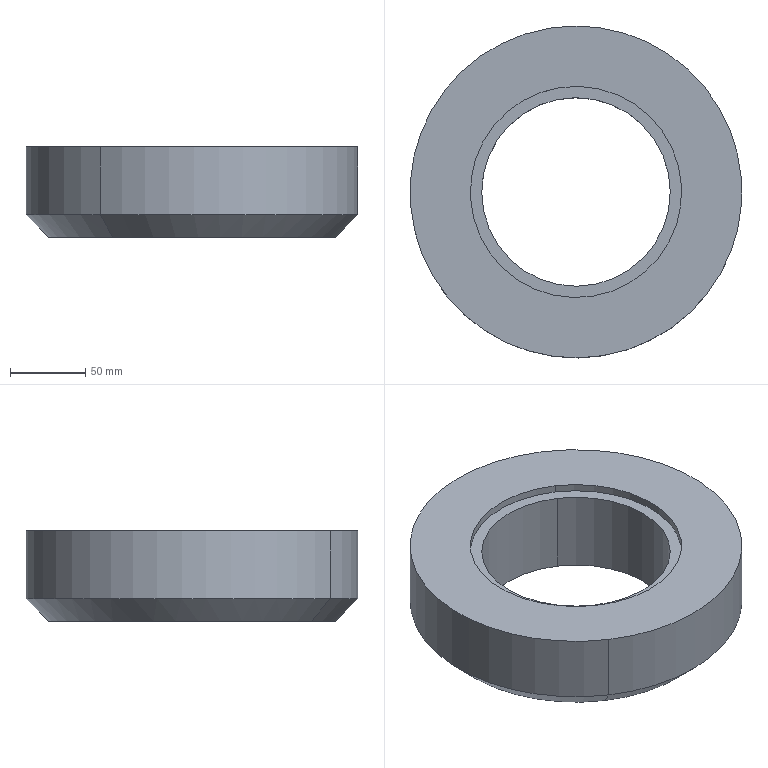Part | SolidWorks | features SplitBody 1 | 1 solid | 11 faces | box 220 x 220 x 60 mm | volume 1454656 mm3 | cylinder 6 | plane 3 | cone 2 | commonest cylinder face diameters 125 x2 140 x2 220 x2
STEP:
#1=CARTESIAN_POINT('',(4251.77,375.62,817.5));
#2=VERTEX_POINT('',#1);
#3=CARTESIAN_POINT('',(4130.11,192.32,817.5));
#4=VERTEX_POINT('',#3);
#5=CARTESIAN_POINT('',(4190.94,283.97,817.5));
#6=DIRECTION('',(0.,0.,1.));
#7=DIRECTION('',(0.553,0.8332,0.));
#8=AXIS2_PLACEMENT_3D('',#5,#6,#7);
#9=CIRCLE('',#8,110.);
#10=EDGE_CURVE('',#2,#4,#9,.T.);
#11=ORIENTED_EDGE('',*,*,#10,.T.);
#12=CARTESIAN_POINT('',(4130.11,192.32,862.5));
#13=VERTEX_POINT('',#12);
#14=CARTESIAN_POINT('',(4130.11,192.32,802.5));
#15=DIRECTION('',(0.,0.,1.));
#16=VECTOR('',#15,1000.);
#17=LINE('',#14,#16);
#18=EDGE_CURVE('',#4,#13,#17,.T.);
#19=ORIENTED_EDGE('',*,*,#18,.T.);
#20=CARTESIAN_POINT('',(4251.77,375.62,862.5));
#21=VERTEX_POINT('',#20);
#22=CARTESIAN_POINT('',(4190.94,283.97,862.5));
#23=DIRECTION('',(0.,0.,-1.));
#24=DIRECTION('',(0.553,0.8332,0.));
#25=AXIS2_PLACEMENT_3D('',#22,#23,#24);
#26=CIRCLE('',#25,110.);
#27=EDGE_CURVE('',#13,#21,#26,.T.);
#28=ORIENTED_EDGE('',*,*,#27,.T.);
#29=CARTESIAN_POINT('',(4251.77,375.62,802.5));
#30=DIRECTION('',(0.,0.,1.));
#31=VECTOR('',#30,1000.);
#32=LINE('',#29,#31);
#33=EDGE_CURVE('',#2,#21,#32,.T.);
#34=ORIENTED_EDGE('',*,*,#33,.F.);
#35=EDGE_LOOP('',(#11,#19,#28,#34));
#36=FACE_OUTER_BOUND('',#35,.T.);
#37=CARTESIAN_POINT('',(4190.94,283.97,802.5));
#38=DIRECTION('',(0.,0.,1.));
#39=DIRECTION('',(0.553,0.8332,0.));
#40=AXIS2_PLACEMENT_3D('',#37,#38,#39);
#41=CYLINDRICAL_SURFACE('',#40,110.);
#42=ADVANCED_FACE('',(#36),#41,.T.);
#43=CARTESIAN_POINT('',(4152.23,225.647,857.5));
#44=VERTEX_POINT('',#43);
#45=CARTESIAN_POINT('',(4229.65,342.293,857.5));
#46=VERTEX_POINT('',#45);
#47=CARTESIAN_POINT('',(4190.94,283.97,857.5));
#48=DIRECTION('',(0.,0.,1.));
#49=DIRECTION('',(0.553,0.8332,0.));
#50=AXIS2_PLACEMENT_3D('',#47,#48,#49);
#51=CIRCLE('',#50,70.);
#52=EDGE_CURVE('',#44,#46,#51,.T.);
#53=ORIENTED_EDGE('',*,*,#52,.F.);
#54=CARTESIAN_POINT('',(4152.23,225.647,862.5));
#55=VERTEX_POINT('',#54);
#56=CARTESIAN_POINT('',(4152.23,225.647,857.5));
#57=DIRECTION('',(0.,0.,1.));
#58=VECTOR('',#57,1000.);
#59=LINE('',#56,#58);
#60=EDGE_CURVE('',#44,#55,#59,.T.);
#61=ORIENTED_EDGE('',*,*,#60,.T.);
#62=CARTESIAN_POINT('',(4229.65,342.293,862.5));
#63=VERTEX_POINT('',#62);
#64=CARTESIAN_POINT('',(4190.94,283.97,862.5));
#65=DIRECTION('',(0.,0.,1.));
#66=DIRECTION('',(0.553,0.8332,0.));
#67=AXIS2_PLACEMENT_3D('',#64,#65,#66);
#68=CIRCLE('',#67,70.);
#69=EDGE_CURVE('',#55,#63,#68,.T.);
#70=ORIENTED_EDGE('',*,*,#69,.T.);
#71=CARTESIAN_POINT('',(4229.65,342.293,857.5));
#72=DIRECTION('',(0.,0.,1.));
#73=VECTOR('',#72,1000.);
#74=LINE('',#71,#73);
#75=EDGE_CURVE('',#46,#63,#74,.T.);
#76=ORIENTED_EDGE('',*,*,#75,.F.);
#77=EDGE_LOOP('',(#53,#61,#70,#76));
#78=FACE_OUTER_BOUND('',#77,.T.);
#79=CARTESIAN_POINT('',(4190.94,283.97,857.5));
#80=DIRECTION('',(0.,0.,1.));
#81=DIRECTION('',(0.553,0.8332,0.));
#82=AXIS2_PLACEMENT_3D('',#79,#80,#81);
#83=CYLINDRICAL_SURFACE('',#82,70.);
#84=ADVANCED_FACE('',(#78),#83,.F.);
#85=CARTESIAN_POINT('',(4243.475,363.122,802.5));
#86=VERTEX_POINT('',#85);
#87=CARTESIAN_POINT('',(4138.405,204.817,802.5));
#88=VERTEX_POINT('',#87);
#89=CARTESIAN_POINT('',(4190.94,283.97,802.5));
#90=DIRECTION('',(0.,0.,1.));
#91=DIRECTION('',(0.553,0.8332,0.));
#92=AXIS2_PLACEMENT_3D('',#89,#90,#91);
#93=CIRCLE('',#92,95.);
#94=EDGE_CURVE('',#86,#88,#93,.T.);
#95=ORIENTED_EDGE('',*,*,#94,.T.);
#96=CARTESIAN_POINT('',(4130.11,192.32,817.5));
#97=DIRECTION('',(-0.391,-0.5891,0.7071));
#98=VECTOR('',#97,1000.);
#99=LINE('',#96,#98);
#100=EDGE_CURVE('',#88,#4,#99,.T.);
#101=ORIENTED_EDGE('',*,*,#100,.T.);
#102=ORIENTED_EDGE('',*,*,#10,.F.);
#103=CARTESIAN_POINT('',(4251.77,375.62,817.5));
#104=DIRECTION('',(0.391,0.5891,0.7071));
#105=VECTOR('',#104,1000.);
#106=LINE('',#103,#105);
#107=EDGE_CURVE('',#86,#2,#106,.T.);
#108=ORIENTED_EDGE('',*,*,#107,.F.);
#109=EDGE_LOOP('',(#95,#101,#102,#108));
#110=FACE_OUTER_BOUND('',#109,.T.);
#111=CARTESIAN_POINT('',(4190.94,283.97,817.5));
#112=DIRECTION('',(0.,0.,1.));
#113=DIRECTION('',(0.553,0.8332,0.));
#114=AXIS2_PLACEMENT_3D('',#111,#112,#113);
#115=CONICAL_SURFACE('',#114,110.,0.7854);
#116=ADVANCED_FACE('',(#110),#115,.T.);
#117=CARTESIAN_POINT('',(4156.378,231.896,802.5));
#118=VERTEX_POINT('',#117);
#119=CARTESIAN_POINT('',(4225.502,336.044,802.5));
#120=VERTEX_POINT('',#119);
#121=CARTESIAN_POINT('',(4190.94,283.97,802.5));
#122=DIRECTION('',(0.,0.,1.));
#123=DIRECTION('',(0.553,0.8332,0.));
#124=AXIS2_PLACEMENT_3D('',#121,#122,#123);
#125=CIRCLE('',#124,62.5);
#126=EDGE_CURVE('',#118,#120,#125,.T.);
#127=ORIENTED_EDGE('',*,*,#126,.F.);
#128=CARTESIAN_POINT('',(4156.378,231.896,857.5));
#129=VERTEX_POINT('',#128);
#130=CARTESIAN_POINT('',(4156.378,231.896,802.5));
#131=DIRECTION('',(0.,0.,1.));
#132=VECTOR('',#131,1000.);
#133=LINE('',#130,#132);
#134=EDGE_CURVE('',#118,#129,#133,.T.);
#135=ORIENTED_EDGE('',*,*,#134,.T.);
#136=CARTESIAN_POINT('',(4225.502,336.044,857.5));
#137=VERTEX_POINT('',#136);
#138=CARTESIAN_POINT('',(4190.94,283.97,857.5));
#139=DIRECTION('',(0.,0.,-1.));
#140=DIRECTION('',(0.553,0.8332,0.));
#141=AXIS2_PLACEMENT_3D('',#138,#139,#140);
#142=CIRCLE('',#141,62.5);
#143=EDGE_CURVE('',#137,#129,#142,.T.);
#144=ORIENTED_EDGE('',*,*,#143,.F.);
#145=CARTESIAN_POINT('',(4225.502,336.044,802.5));
#146=DIRECTION('',(0.,0.,1.));
#147=VECTOR('',#146,1000.);
#148=LINE('',#145,#147);
#149=EDGE_CURVE('',#120,#137,#148,.T.);
#150=ORIENTED_EDGE('',*,*,#149,.F.);
#151=EDGE_LOOP('',(#127,#135,#144,#150));
#152=FACE_OUTER_BOUND('',#151,.T.);
#153=CARTESIAN_POINT('',(4190.94,283.97,802.5));
#154=DIRECTION('',(0.,0.,1.));
#155=DIRECTION('',(0.553,0.8332,0.));
#156=AXIS2_PLACEMENT_3D('',#153,#154,#155);
#157=CYLINDRICAL_SURFACE('',#156,62.5);
#158=ADVANCED_FACE('',(#152),#157,.F.);
#159=CARTESIAN_POINT('',(4190.94,283.97,862.5));
#160=DIRECTION('',(0.,0.,-1.));
#161=DIRECTION('',(0.553,0.8332,0.));
#162=AXIS2_PLACEMENT_3D('',#159,#160,#161);
#163=CIRCLE('',#162,110.);
#164=EDGE_CURVE('',#21,#13,#163,.T.);
#165=ORIENTED_EDGE('',*,*,#164,.F.);
#166=ORIENTED_EDGE('',*,*,#27,.F.);
#167=EDGE_LOOP('',(#165,#166));
#168=FACE_OUTER_BOUND('',#167,.T.);
#169=CARTESIAN_POINT('',(4190.94,283.97,862.5));
#170=DIRECTION('',(0.,0.,1.));
#171=DIRECTION('',(0.553,0.8332,0.));
#172=AXIS2_PLACEMENT_3D('',#169,#170,#171);
#173=CIRCLE('',#172,70.);
#174=EDGE_CURVE('',#63,#55,#173,.T.);
#175=ORIENTED_EDGE('',*,*,#174,.F.);
#176=ORIENTED_EDGE('',*,*,#69,.F.);
#177=EDGE_LOOP('',(#175,#176));
#178=FACE_BOUND('',#177,.T.);
#179=CARTESIAN_POINT('',(4190.94,283.97,862.5));
#180=DIRECTION('',(0.,0.,-1.));
#181=DIRECTION('',(-0.553,-0.8332,0.));
#182=AXIS2_PLACEMENT_3D('',#179,#180,#181);
#183=PLANE('',#182);
#184=ADVANCED_FACE('',(#168,#178),#183,.F.);
#185=ORIENTED_EDGE('',*,*,#18,.F.);
#186=CARTESIAN_POINT('',(4190.94,283.97,817.5));
#187=DIRECTION('',(0.,0.,1.));
#188=DIRECTION('',(0.553,0.8332,0.));
#189=AXIS2_PLACEMENT_3D('',#186,#187,#188);
#190=CIRCLE('',#189,110.);
#191=EDGE_CURVE('',#4,#2,#190,.T.);
#192=ORIENTED_EDGE('',*,*,#191,.T.);
#193=ORIENTED_EDGE('',*,*,#33,.T.);
#194=ORIENTED_EDGE('',*,*,#164,.T.);
#195=EDGE_LOOP('',(#185,#192,#193,#194));
#196=FACE_OUTER_BOUND('',#195,.T.);
#197=CARTESIAN_POINT('',(4190.94,283.97,802.5));
#198=DIRECTION('',(0.,0.,1.));
#199=DIRECTION('',(0.553,0.8332,0.));
#200=AXIS2_PLACEMENT_3D('',#197,#198,#199);
#201=CYLINDRICAL_SURFACE('',#200,110.);
#202=ADVANCED_FACE('',(#196),#201,.T.);
#203=ORIENTED_EDGE('',*,*,#60,.F.);
#204=CARTESIAN_POINT('',(4190.94,283.97,857.5));
#205=DIRECTION('',(0.,0.,1.));
#206=DIRECTION('',(0.553,0.8332,0.));
#207=AXIS2_PLACEMENT_3D('',#204,#205,#206);
#208=CIRCLE('',#207,70.);
#209=EDGE_CURVE('',#46,#44,#208,.T.);
#210=ORIENTED_EDGE('',*,*,#209,.F.);
#211=ORIENTED_EDGE('',*,*,#75,.T.);
#212=ORIENTED_EDGE('',*,*,#174,.T.);
#213=EDGE_LOOP('',(#203,#210,#211,#212));
#214=FACE_OUTER_BOUND('',#213,.T.);
#215=CARTESIAN_POINT('',(4190.94,283.97,857.5));
#216=DIRECTION('',(0.,0.,1.));
#217=DIRECTION('',(0.553,0.8332,0.));
#218=AXIS2_PLACEMENT_3D('',#215,#216,#217);
#219=CYLINDRICAL_SURFACE('',#218,70.);
#220=ADVANCED_FACE('',(#214),#219,.F.);
#221=ORIENTED_EDGE('',*,*,#100,.F.);
#222=CARTESIAN_POINT('',(4190.94,283.97,802.5));
#223=DIRECTION('',(0.,0.,1.));
#224=DIRECTION('',(0.553,0.8332,0.));
#225=AXIS2_PLACEMENT_3D('',#222,#223,#224);
#226=CIRCLE('',#225,95.);
#227=EDGE_CURVE('',#88,#86,#226,.T.);
#228=ORIENTED_EDGE('',*,*,#227,.T.);
#229=ORIENTED_EDGE('',*,*,#107,.T.);
#230=ORIENTED_EDGE('',*,*,#191,.F.);
#231=EDGE_LOOP('',(#221,#228,#229,#230));
#232=FACE_OUTER_BOUND('',#231,.T.);
#233=CARTESIAN_POINT('',(4190.94,283.97,817.5));
#234=DIRECTION('',(0.,0.,1.));
#235=DIRECTION('',(0.553,0.8332,0.));
#236=AXIS2_PLACEMENT_3D('',#233,#234,#235);
#237=CONICAL_SURFACE('',#236,110.,0.7854);
#238=ADVANCED_FACE('',(#232),#237,.T.);
#239=ORIENTED_EDGE('',*,*,#209,.T.);
#240=ORIENTED_EDGE('',*,*,#52,.T.);
#241=EDGE_LOOP('',(#239,#240));
#242=FACE_OUTER_BOUND('',#241,.T.);
#243=ORIENTED_EDGE('',*,*,#143,.T.);
#244=CARTESIAN_POINT('',(4190.94,283.97,857.5));
#245=DIRECTION('',(0.,0.,-1.));
#246=DIRECTION('',(0.553,0.8332,0.));
#247=AXIS2_PLACEMENT_3D('',#244,#245,#246);
#248=CIRCLE('',#247,62.5);
#249=EDGE_CURVE('',#129,#137,#248,.T.);
#250=ORIENTED_EDGE('',*,*,#249,.T.);
#251=EDGE_LOOP('',(#243,#250));
#252=FACE_BOUND('',#251,.T.);
#253=CARTESIAN_POINT('',(4190.94,283.97,857.5));
#254=DIRECTION('',(0.,0.,1.));
#255=DIRECTION('',(0.553,0.8332,0.));
#256=AXIS2_PLACEMENT_3D('',#253,#254,#255);
#257=PLANE('',#256);
#258=ADVANCED_FACE('',(#242,#252),#257,.T.);
#259=CARTESIAN_POINT('',(4190.94,283.97,802.5));
#260=DIRECTION('',(0.,0.,1.));
#261=DIRECTION('',(0.553,0.8332,0.));
#262=AXIS2_PLACEMENT_3D('',#259,#260,#261);
#263=CIRCLE('',#262,62.5);
#264=EDGE_CURVE('',#120,#118,#263,.T.);
#265=ORIENTED_EDGE('',*,*,#264,.T.);
#266=ORIENTED_EDGE('',*,*,#126,.T.);
#267=EDGE_LOOP('',(#265,#266));
#268=FACE_BOUND('',#267,.T.);
#269=ORIENTED_EDGE('',*,*,#94,.F.);
#270=ORIENTED_EDGE('',*,*,#227,.F.);
#271=EDGE_LOOP('',(#269,#270));
#272=FACE_OUTER_BOUND('',#271,.T.);
#273=CARTESIAN_POINT('',(4190.94,283.97,802.5));
#274=DIRECTION('',(0.,0.,-1.));
#275=DIRECTION('',(-0.553,-0.8332,0.));
#276=AXIS2_PLACEMENT_3D('',#273,#274,#275);
#277=PLANE('',#276);
#278=ADVANCED_FACE('',(#268,#272),#277,.T.);
#279=ORIENTED_EDGE('',*,*,#134,.F.);
#280=ORIENTED_EDGE('',*,*,#264,.F.);
#281=ORIENTED_EDGE('',*,*,#149,.T.);
#282=ORIENTED_EDGE('',*,*,#249,.F.);
#283=EDGE_LOOP('',(#279,#280,#281,#282));
#284=FACE_OUTER_BOUND('',#283,.T.);
#285=CARTESIAN_POINT('',(4190.94,283.97,802.5));
#286=DIRECTION('',(0.,0.,1.));
#287=DIRECTION('',(0.553,0.8332,0.));
#288=AXIS2_PLACEMENT_3D('',#285,#286,#287);
#289=CYLINDRICAL_SURFACE('',#288,62.5);
#290=ADVANCED_FACE('',(#284),#289,.F.);
#291=CLOSED_SHELL('',(#42,#84,#116,#158,#184,#202,#220,#238,#258,#278,#290));
#292=MANIFOLD_SOLID_BREP('',#291);
#293=CARTESIAN_POINT('',(0.,0.,0.));
#294=DIRECTION('',(0.,0.,1.));
#295=DIRECTION('',(1.,0.,0.));
#296=AXIS2_PLACEMENT_3D('',#293,#294,#295);
#297=(LENGTH_UNIT()NAMED_UNIT(*)SI_UNIT(.MILLI.,.METRE.));
#298=UNCERTAINTY_MEASURE_WITH_UNIT(LENGTH_MEASURE(0.00001),#297,'','');
#299=(NAMED_UNIT(*)PLANE_ANGLE_UNIT()SI_UNIT($,.RADIAN.));
#300=(NAMED_UNIT(*)SI_UNIT($,.STERADIAN.)SOLID_ANGLE_UNIT());
#301=(GEOMETRIC_REPRESENTATION_CONTEXT(3)GLOBAL_UNCERTAINTY_ASSIGNED_CONTEXT((#298))GLOBAL_UNIT_ASSIGNED_CONTEXT((#297,#299,#300))REPRESENTATION_CONTEXT('',''));
#302=ADVANCED_BREP_SHAPE_REPRESENTATION('',(#292,#296),#301);